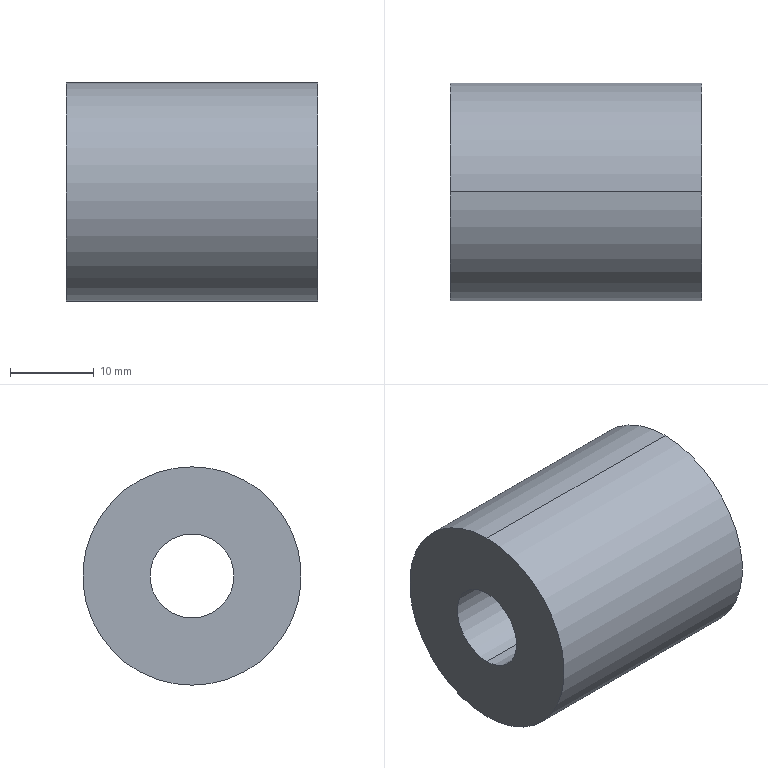Part | SolidWorks | features BaseBody 1 | 1 solid | 6 faces | box 30 x 26 x 26 mm | volume 13572 mm3 | cylinder 4 | plane 2 | commonest cylinder face diameters 10 x2 26 x2
STEP:
#1=CARTESIAN_POINT('',(104.,-57.,-6.));
#2=VERTEX_POINT('',#1);
#3=CARTESIAN_POINT('',(104.,-57.,20.));
#4=VERTEX_POINT('',#3);
#5=CARTESIAN_POINT('',(104.,-57.,7.));
#6=DIRECTION('',(1.,0.,0.));
#7=DIRECTION('',(0.,0.,-1.));
#8=AXIS2_PLACEMENT_3D('',#5,#6,#7);
#9=CIRCLE('',#8,13.);
#10=EDGE_CURVE('',#2,#4,#9,.T.);
#11=ORIENTED_EDGE('',*,*,#10,.T.);
#12=CARTESIAN_POINT('',(134.,-57.,20.));
#13=VERTEX_POINT('',#12);
#14=CARTESIAN_POINT('',(104.,-57.,20.));
#15=DIRECTION('',(1.,0.,0.));
#16=VECTOR('',#15,1000.);
#17=LINE('',#14,#16);
#18=EDGE_CURVE('',#4,#13,#17,.T.);
#19=ORIENTED_EDGE('',*,*,#18,.T.);
#20=CARTESIAN_POINT('',(134.,-57.,-6.));
#21=VERTEX_POINT('',#20);
#22=CARTESIAN_POINT('',(134.,-57.,7.));
#23=DIRECTION('',(-1.,0.,0.));
#24=DIRECTION('',(0.,0.,-1.));
#25=AXIS2_PLACEMENT_3D('',#22,#23,#24);
#26=CIRCLE('',#25,13.);
#27=EDGE_CURVE('',#13,#21,#26,.T.);
#28=ORIENTED_EDGE('',*,*,#27,.T.);
#29=CARTESIAN_POINT('',(104.,-57.,-6.));
#30=DIRECTION('',(1.,0.,0.));
#31=VECTOR('',#30,1000.);
#32=LINE('',#29,#31);
#33=EDGE_CURVE('',#2,#21,#32,.T.);
#34=ORIENTED_EDGE('',*,*,#33,.F.);
#35=EDGE_LOOP('',(#11,#19,#28,#34));
#36=FACE_OUTER_BOUND('',#35,.T.);
#37=CARTESIAN_POINT('',(104.,-57.,7.));
#38=DIRECTION('',(1.,0.,0.));
#39=DIRECTION('',(0.,0.,-1.));
#40=AXIS2_PLACEMENT_3D('',#37,#38,#39);
#41=CYLINDRICAL_SURFACE('',#40,13.);
#42=ADVANCED_FACE('',(#36),#41,.T.);
#43=CARTESIAN_POINT('',(104.,-57.,2.));
#44=VERTEX_POINT('',#43);
#45=CARTESIAN_POINT('',(104.,-57.,12.));
#46=VERTEX_POINT('',#45);
#47=CARTESIAN_POINT('',(104.,-57.,7.));
#48=DIRECTION('',(-1.,0.,0.));
#49=DIRECTION('',(0.,0.,-1.));
#50=AXIS2_PLACEMENT_3D('',#47,#48,#49);
#51=CIRCLE('',#50,5.);
#52=EDGE_CURVE('',#44,#46,#51,.T.);
#53=ORIENTED_EDGE('',*,*,#52,.T.);
#54=CARTESIAN_POINT('',(134.,-57.,12.));
#55=VERTEX_POINT('',#54);
#56=CARTESIAN_POINT('',(104.,-57.,12.));
#57=DIRECTION('',(1.,0.,0.));
#58=VECTOR('',#57,1000.);
#59=LINE('',#56,#58);
#60=EDGE_CURVE('',#46,#55,#59,.T.);
#61=ORIENTED_EDGE('',*,*,#60,.T.);
#62=CARTESIAN_POINT('',(134.,-57.,2.));
#63=VERTEX_POINT('',#62);
#64=CARTESIAN_POINT('',(134.,-57.,7.));
#65=DIRECTION('',(-1.,0.,0.));
#66=DIRECTION('',(0.,0.,-1.));
#67=AXIS2_PLACEMENT_3D('',#64,#65,#66);
#68=CIRCLE('',#67,5.);
#69=EDGE_CURVE('',#63,#55,#68,.T.);
#70=ORIENTED_EDGE('',*,*,#69,.F.);
#71=CARTESIAN_POINT('',(104.,-57.,2.));
#72=DIRECTION('',(1.,0.,0.));
#73=VECTOR('',#72,1000.);
#74=LINE('',#71,#73);
#75=EDGE_CURVE('',#44,#63,#74,.T.);
#76=ORIENTED_EDGE('',*,*,#75,.F.);
#77=EDGE_LOOP('',(#53,#61,#70,#76));
#78=FACE_OUTER_BOUND('',#77,.T.);
#79=CARTESIAN_POINT('',(104.,-57.,7.));
#80=DIRECTION('',(1.,0.,0.));
#81=DIRECTION('',(0.,0.,-1.));
#82=AXIS2_PLACEMENT_3D('',#79,#80,#81);
#83=CYLINDRICAL_SURFACE('',#82,5.);
#84=ADVANCED_FACE('',(#78),#83,.F.);
#85=ORIENTED_EDGE('',*,*,#18,.F.);
#86=CARTESIAN_POINT('',(104.,-57.,7.));
#87=DIRECTION('',(1.,0.,0.));
#88=DIRECTION('',(0.,0.,-1.));
#89=AXIS2_PLACEMENT_3D('',#86,#87,#88);
#90=CIRCLE('',#89,13.);
#91=EDGE_CURVE('',#4,#2,#90,.T.);
#92=ORIENTED_EDGE('',*,*,#91,.T.);
#93=ORIENTED_EDGE('',*,*,#33,.T.);
#94=CARTESIAN_POINT('',(134.,-57.,7.));
#95=DIRECTION('',(-1.,0.,0.));
#96=DIRECTION('',(0.,0.,-1.));
#97=AXIS2_PLACEMENT_3D('',#94,#95,#96);
#98=CIRCLE('',#97,13.);
#99=EDGE_CURVE('',#21,#13,#98,.T.);
#100=ORIENTED_EDGE('',*,*,#99,.T.);
#101=EDGE_LOOP('',(#85,#92,#93,#100));
#102=FACE_OUTER_BOUND('',#101,.T.);
#103=CARTESIAN_POINT('',(104.,-57.,7.));
#104=DIRECTION('',(1.,0.,0.));
#105=DIRECTION('',(0.,0.,-1.));
#106=AXIS2_PLACEMENT_3D('',#103,#104,#105);
#107=CYLINDRICAL_SURFACE('',#106,13.);
#108=ADVANCED_FACE('',(#102),#107,.T.);
#109=ORIENTED_EDGE('',*,*,#52,.F.);
#110=CARTESIAN_POINT('',(104.,-57.,7.));
#111=DIRECTION('',(-1.,0.,0.));
#112=DIRECTION('',(0.,0.,-1.));
#113=AXIS2_PLACEMENT_3D('',#110,#111,#112);
#114=CIRCLE('',#113,5.);
#115=EDGE_CURVE('',#46,#44,#114,.T.);
#116=ORIENTED_EDGE('',*,*,#115,.F.);
#117=EDGE_LOOP('',(#109,#116));
#118=FACE_BOUND('',#117,.T.);
#119=ORIENTED_EDGE('',*,*,#10,.F.);
#120=ORIENTED_EDGE('',*,*,#91,.F.);
#121=EDGE_LOOP('',(#119,#120));
#122=FACE_OUTER_BOUND('',#121,.T.);
#123=CARTESIAN_POINT('',(104.,-57.,7.));
#124=DIRECTION('',(1.,0.,0.));
#125=DIRECTION('',(0.,0.,-1.));
#126=AXIS2_PLACEMENT_3D('',#123,#124,#125);
#127=PLANE('',#126);
#128=ADVANCED_FACE('',(#118,#122),#127,.F.);
#129=ORIENTED_EDGE('',*,*,#69,.T.);
#130=CARTESIAN_POINT('',(134.,-57.,7.));
#131=DIRECTION('',(-1.,0.,0.));
#132=DIRECTION('',(0.,0.,-1.));
#133=AXIS2_PLACEMENT_3D('',#130,#131,#132);
#134=CIRCLE('',#133,5.);
#135=EDGE_CURVE('',#55,#63,#134,.T.);
#136=ORIENTED_EDGE('',*,*,#135,.T.);
#137=EDGE_LOOP('',(#129,#136));
#138=FACE_BOUND('',#137,.T.);
#139=ORIENTED_EDGE('',*,*,#99,.F.);
#140=ORIENTED_EDGE('',*,*,#27,.F.);
#141=EDGE_LOOP('',(#139,#140));
#142=FACE_OUTER_BOUND('',#141,.T.);
#143=CARTESIAN_POINT('',(134.,-57.,7.));
#144=DIRECTION('',(1.,0.,0.));
#145=DIRECTION('',(0.,0.,-1.));
#146=AXIS2_PLACEMENT_3D('',#143,#144,#145);
#147=PLANE('',#146);
#148=ADVANCED_FACE('',(#138,#142),#147,.T.);
#149=ORIENTED_EDGE('',*,*,#60,.F.);
#150=ORIENTED_EDGE('',*,*,#115,.T.);
#151=ORIENTED_EDGE('',*,*,#75,.T.);
#152=ORIENTED_EDGE('',*,*,#135,.F.);
#153=EDGE_LOOP('',(#149,#150,#151,#152));
#154=FACE_OUTER_BOUND('',#153,.T.);
#155=CARTESIAN_POINT('',(104.,-57.,7.));
#156=DIRECTION('',(1.,0.,0.));
#157=DIRECTION('',(0.,0.,-1.));
#158=AXIS2_PLACEMENT_3D('',#155,#156,#157);
#159=CYLINDRICAL_SURFACE('',#158,5.);
#160=ADVANCED_FACE('',(#154),#159,.F.);
#161=CLOSED_SHELL('',(#42,#84,#108,#128,#148,#160));
#162=MANIFOLD_SOLID_BREP('',#161);
#163=CARTESIAN_POINT('',(0.,0.,0.));
#164=DIRECTION('',(0.,0.,1.));
#165=DIRECTION('',(1.,0.,0.));
#166=AXIS2_PLACEMENT_3D('',#163,#164,#165);
#167=(LENGTH_UNIT()NAMED_UNIT(*)SI_UNIT(.MILLI.,.METRE.));
#168=UNCERTAINTY_MEASURE_WITH_UNIT(LENGTH_MEASURE(0.00001),#167,'','');
#169=(NAMED_UNIT(*)PLANE_ANGLE_UNIT()SI_UNIT($,.RADIAN.));
#170=(NAMED_UNIT(*)SI_UNIT($,.STERADIAN.)SOLID_ANGLE_UNIT());
#171=(GEOMETRIC_REPRESENTATION_CONTEXT(3)GLOBAL_UNCERTAINTY_ASSIGNED_CONTEXT((#168))GLOBAL_UNIT_ASSIGNED_CONTEXT((#167,#169,#170))REPRESENTATION_CONTEXT('',''));
#172=ADVANCED_BREP_SHAPE_REPRESENTATION('',(#162,#166),#171);